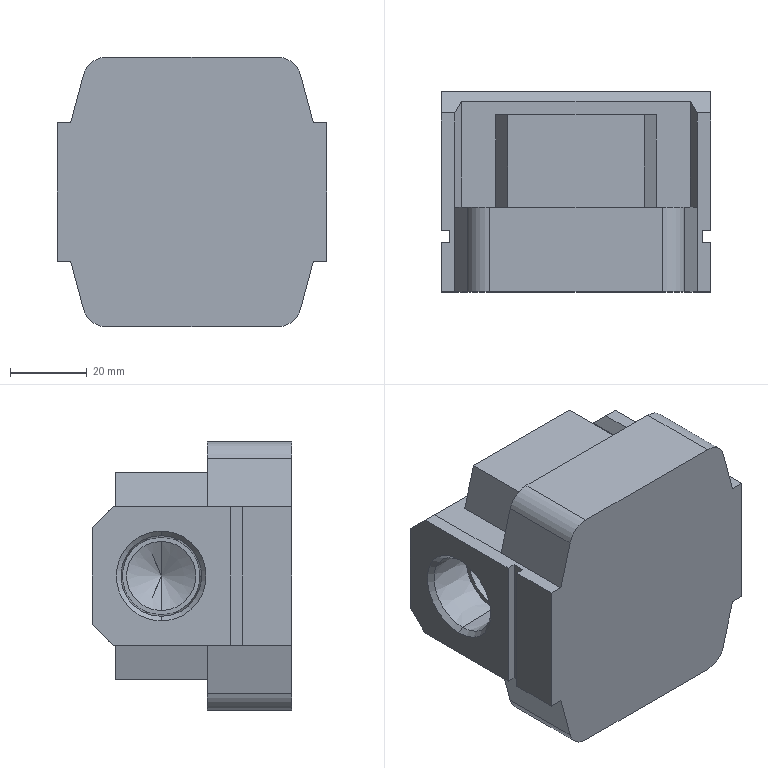Part | STEP file | AC40-04-KSTV-38JNR_AC3009A AF Body-1 | 1 solid | 102 faces | box 70 x 52 x 70 mm | volume 171815 mm3 | plane 50 | cone 28 | cylinder 24 | commonest cylinder face diameters 4.2 x8 5 x8 12 x4 18 x4